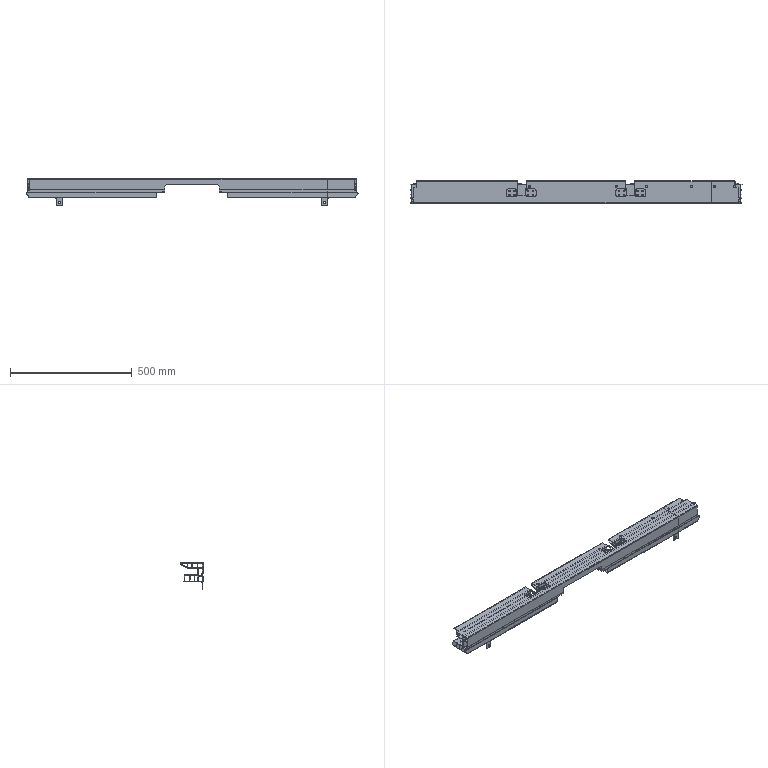NC program | NX | posted with a generic post | part box 1365 x 90.95 x 108.501 mm
Lines 10674 to 11425 of 22311:
(DRILLING , TOOL : D6A45)
N21340 T07 M6
N21342 G54
N21344 G17 G0 G90 X636.499 Y-0.225 B0. C0. S3500 M3
N21346 G43 Z30. H7
N21348 G94 G81 G98 Z-31. F250. R-27.
N21350 X600. Y0.175
N21352 X563.5
N21354 X423. Y0.725
N21356 X373.
N21358 X364.736 Y-18.525
N21360 X328. Y0.725
N21362 X314.736 Y-18.525
N21364 X278. Y0.725
N21366 X264.736 Y-18.525
N21368 X248. Y0.725
N21370 X-248.
N21372 X-264.736 Y-18.525
N21374 X-278. Y0.725
N21376 X-314.736 Y-18.525
N21378 X-328. Y0.725
N21380 X-364.736 Y-18.525
N21382 X-373. Y0.725
N21384 X-423.
N21386 X-563.501 Y-0.225
N21388 X-600. Y0.175
N21390 X-636.5
N21392 G80
N21394 G0 X-636.5 Y0.175 Z30.
(DRILLING_COPY_1 , TOOL : D6A45)
N21396 X25.103 Y-6.202
N21398 G81 Z-86.5 F250. R-82.5
N21400 G80
N21402 G0 X25.103 Y-6.202 Z30.
N21404 M5
(DRILLING_COPY , TOOL : 7.1ZT)
N21406 T17 M6
N21408 G54
N21410 G17 G0 G90 X-636.5 Y0.175 B0. C0. S1500 M3
N21412 G43 Z30. H17
N21414 G94 G83 G98 Z-36.103 F150. Q4. R-27.
N21416 X-563.501 Y-0.225
N21418 X563.5 Y0.175
N21420 X636.499 Y-0.225
N21422 G80
N21424 G0 X636.499 Y-0.225 Z30.
N21426 M5
(DRILLING_COPY_COPY , TOOL : 9.0ZT)
N21428 T19 M6
N21430 G54
N21432 G17 G0 G90 X-423. Y0.725 B0. C0. S1500 M3
N21434 G43 Z30. H19
N21436 G94 G83 G98 Z-36.704 F150. Q4. R-27.
N21438 X-373.
N21440 X-364.736 Y-18.525
N21442 X-328. Y0.725
N21444 X-314.736 Y-18.525
N21446 X-278. Y0.725
N21448 X-264.736 Y-18.525
N21450 X-248. Y0.725
N21452 X248.
N21454 X264.736 Y-18.525
N21456 X278. Y0.725
N21458 X314.736 Y-18.525
N21460 X328. Y0.725
N21462 X364.736 Y-18.525
N21464 X373. Y0.725
N21466 X423.
N21468 G80
N21470 G0 X423. Y0.725 Z30.
N21472 M5
(DRILLING_COPY_COPY_COPY , TOOL : 6.6ZT)
N21474 T14 M6
N21476 G54
N21478 G17 G0 G90 X25.103 Y-6.202 B0. C0. S1500 M3
N21480 G43 Z30. H14
N21482 G94 G83 G98 Z-91.453 F150. Q4. R-82.5
N21484 G80
N21486 G0 X25.103 Y-6.202 Z30.
N21488 M5
(FLOOR_WALL , TOOL : D10)
N21490 T10 M6
N21492 G54
N21494 G17 G0 G90 X-138.045 Y42.675 B0. C0. S6000 M3
N21496 G43 Z30. H10
N21498 Z-28.5
N21500 G94 G1 Z-30. F1000.
N21502 X-140.411 Y41.678
N21504 G3 X-139.545 Y41.178 R1.
N21506 G1 X-522.999
N21508 Y41.234
N21510 X-139.545
N21512 Y41.291
N21514 X-522.999
N21516 Y41.347
N21518 X-139.545
N21520 Y41.403
N21522 X-522.999
N21524 Y41.46
N21526 X-139.545
N21528 Y41.516
N21530 X-522.999
N21532 Y41.572
N21534 X-139.545
N21536 Y41.629
N21538 X-522.999
N21540 Y41.685
N21542 X-139.545
N21544 Y41.741
N21546 X-522.999
N21548 Y41.798
N21550 X-139.545
N21552 Y41.854
N21554 X-522.999
N21556 Y41.91
N21558 X-139.545
N21560 Y41.966
N21562 X-522.999
N21564 Y42.023
N21566 X-139.545
N21568 Y42.079
N21570 X-522.999
N21572 Y42.135
N21574 X-139.545
N21576 Y42.192
N21578 X-522.999
N21580 Y42.248
N21582 X-139.545
N21584 Y42.304
N21586 X-522.999
N21588 Y42.361
N21590 X-139.545
N21592 Y42.417
N21594 X-522.999
N21596 Y42.473
N21598 X-139.545
N21600 Y42.53
N21602 X-522.999
N21604 Y42.586
N21606 X-139.545
N21608 Y42.642
N21610 X-522.999
N21612 Y42.699
N21614 X-139.545
N21616 Y42.755
N21618 X-522.999
N21620 Y42.811
N21622 X-139.545
N21624 Y42.868
N21626 X-522.999
N21628 Y42.924
N21630 X-139.545
N21632 Y42.98
N21634 X-522.999
N21636 Y43.037
N21638 X-139.545
N21640 Y43.093
N21642 X-522.999
N21644 Y43.149
N21646 X-139.545
N21648 Y43.205
N21650 X-522.999
N21652 Y43.262
N21654 X-139.545
N21656 Y43.318
N21658 X-522.999
N21660 Y43.374
N21662 X-139.545
N21664 Y43.431
N21666 X-522.999
N21668 Y43.487
N21670 X-139.545
N21672 Y43.543
N21674 X-522.999
N21676 Y43.6
N21678 X-139.545
N21680 Y43.656
N21682 X-522.999
N21684 Y43.712
N21686 X-139.545
N21688 Y43.769
N21690 X-522.999
N21692 Y43.825
N21694 X-139.545
N21696 Y43.881
N21698 X-522.999
N21700 Y43.938
N21702 X-139.545
N21704 Y43.994
N21706 X-522.999
N21708 Y44.05
N21710 X-139.545
N21712 Y44.107
N21714 X-522.999
N21716 Y44.163
N21718 X-139.545
N21720 Y44.219
N21722 X-522.999
N21724 Y44.276
N21726 X-139.545
N21728 Y44.332
N21730 X-522.999
N21732 Y44.388
N21734 X-139.545
N21736 Y44.445
N21738 X-522.999
N21740 Y44.501
N21742 X-139.545
N21744 Y44.557
N21746 X-522.999
N21748 Y44.613
N21750 X-139.545
N21752 Y44.67
N21754 X-522.999
N21756 Y44.726
N21758 X-139.545
N21760 Y44.782
N21762 X-522.999
N21764 Y44.839
N21766 X-139.545
N21768 Y44.895
N21770 X-522.999
N21772 Y44.951
N21774 X-139.545
N21776 Y45.008
N21778 X-522.999
N21780 Y45.064
N21782 X-139.545
N21784 Y45.12
N21786 X-522.999
N21788 Y45.177
N21790 X-139.545
N21792 Y45.233
N21794 X-522.999
N21796 G3 X-522.499 Y44.367 R1.
N21798 G1 Z-28.5
N21800 G0 Z30.
N21802 X-674.702 Y46.829
N21804 Z-28.5
N21806 G1 Z-30.
N21808 X-674.068 Y45.731
N21810 G3 X-673.202 Y45.231 R1.
N21812 G1 X-566.999
N21814 Y41.175
N21816 X-673.202
N21818 G2 X-674.068 Y41.675 R1.
N21820 G1 X-674.702 Y42.773
N21822 Z-28.5
N21824 G0 Z30.
N21826 X138.164 Y46.627
N21828 Z-28.5
N21830 G1 Z-30.
N21832 X138.681 Y45.731
N21834 G3 X139.547 Y45.231 R1.
N21836 G1 X523.001
N21838 Y41.175
N21840 X139.547
N21842 G2 X138.681 Y41.675 R1.
N21844 G1 X138.047 Y42.773
N21846 Z-28.5
N21848 G0 Z30.
(FLOOR_WALL_COPY , TOOL : D10)
N21850 X110.406 Y15.475
N21852 Z-51.5
N21854 G1 Z-53.
N21856 X111.504 Y16.109
N21858 G3 X112.004 Y16.975 R1.
N21860 G1 Y47.475
N21862 X116.511
N21864 Y16.975
N21866 X121.018
N21868 Y48.975
N21870 X125.525
N21872 Y16.975
N21874 X130.033
N21876 Y48.975
N21878 X134.54
N21880 Y16.975
N21882 X139.047
N21884 Y48.975
N21886 G3 X138.547 Y49.841 R1.
N21888 G1 X137.449 Y50.475
N21890 Z-51.5
N21892 G0 Z30.
N21894 X137.949 Y15.475
N21896 Z-51.5
N21898 G1 Z-53.
N21900 X139.047 Y16.109
N21902 G3 X139.547 Y16.975 R1.
N21904 G1 Y46.046
N21906 X142.303 Y48.801
N21908 X142.451 Y48.945
N21910 G3 X142.727 Y49.906 R1.
N21912 G1 X142.453 Y51.007
N21914 Z-51.5
N21916 G0 Z30.
N21918 X95.501 Y34.652
N21920 Z-83.5
N21922 G1 Z-85.
N21924 X95.998 Y32.286
N21926 G3 X96.498 Y33.152 R1.
N21928 G1 Y17.798
N21930 X91.549
N21932 Y33.152
N21934 X86.601
N21936 Y17.798
N21938 X81.652
N21940 Y33.152
N21942 X76.703
N21944 Y17.798
N21946 X71.755
N21948 Y33.152
N21950 X66.806
N21952 Y17.798
N21954 X61.857
N21956 Y33.152
N21958 X56.909
N21960 Y17.798
N21962 X51.96
N21964 Y33.152
N21966 X47.011
N21968 Y17.798
N21970 X42.063
N21972 Y33.152
N21974 X37.114
N21976 Y17.798
N21978 X32.166
N21980 Y33.152
N21982 X27.217
N21984 Y17.798
N21986 X22.268
N21988 Y33.152
N21990 X17.32
N21992 Y17.798
N21994 X12.371
N21996 Y33.152
N21998 X7.422
N22000 Y17.798
N22002 X2.474
N22004 Y33.152
N22006 X-2.475
N22008 Y17.798
N22010 X-7.424
N22012 Y33.152
N22014 X-12.372
N22016 Y17.798
N22018 X-17.321
N22020 Y33.152
N22022 X-22.269
N22024 Y17.798
N22026 X-27.218
N22028 Y33.152
N22030 X-32.167
N22032 Y17.798
N22034 X-37.115
N22036 Y33.152
N22038 X-42.064
N22040 Y17.798
N22042 X-47.013
N22044 Y33.152
N22046 X-51.961
N22048 Y17.798
N22050 X-56.91
N22052 Y33.152
N22054 X-61.859
N22056 Y17.798
N22058 X-66.807
N22060 Y33.152
N22062 X-71.756
N22064 Y17.798
N22066 X-76.705
N22068 Y33.152
N22070 X-81.653
N22072 Y17.798
N22074 X-86.602
N22076 Y33.152
N22078 X-91.55
N22080 Y17.798
N22082 X-96.499
N22084 Y33.152
N22086 G2 X-95.999 Y34.018 R1.
N22088 G1 X-94.901 Y34.652
N22090 Z-83.5
N22092 G0 Z30.
N22094 X-95.401
N22096 Z-83.5
N22098 G1 Z-85.
N22100 X-96.499 Y34.018
N22102 G3 X-96.999 Y33.152 R1.
N22104 G1 Y17.798
N22106 G3 X-96.499 Y16.932 R1.
N22108 G1 X-95.401 Y16.298
N22110 Z-83.5
N22112 G0 Z30.
N22114 X95.403
N22116 Z-83.5
N22118 G1 Z-85.
N22120 X96.501 Y16.932
N22122 G3 X97.001 Y17.798 R1.
N22124 G1 Y33.152
N22126 G3 X96.501 Y34.018 R1.
N22128 G1 X95.403 Y34.652
N22130 Z-83.5
N22132 G0 Z30.
N22134 X95.998 Y51.975
N22136 Z-83.5
N22138 G1 Z-85.
N22140 Y49.609
N22142 G3 X96.498 Y50.475 R1.
N22144 G1 Y35.798
N22146 X91.549
N22148 Y50.475
N22150 X86.601
N22152 Y35.798
N22154 X81.652
N22156 Y50.475
N22158 X76.703
N22160 Y35.798
N22162 X71.755
N22164 Y50.475
N22166 X66.806
N22168 Y35.798
N22170 X61.857
N22172 Y50.475
N22174 X56.909
N22176 Y35.798
N22178 X51.96
N22180 Y50.475
N22182 X47.011
N22184 Y35.798
N22186 X42.063
N22188 Y50.475
N22190 X37.114
N22192 Y35.798
N22194 X32.166
N22196 Y50.475
N22198 X27.217
N22200 Y35.798
N22202 X22.268
N22204 Y50.475
N22206 X17.32
N22208 Y35.798
N22210 X12.371
N22212 Y50.475
N22214 X7.422
N22216 Y35.798
N22218 X2.474
N22220 Y50.475
N22222 X-2.475
N22224 Y35.798
N22226 X-7.424
N22228 Y50.475
N22230 X-12.372
N22232 Y35.798
N22234 X-17.321
N22236 Y50.475
N22238 X-22.269
N22240 Y35.798
N22242 X-27.218
N22244 Y50.475
N22246 X-32.167
N22248 Y35.798
N22250 X-37.115
N22252 Y50.475
N22254 X-42.064
N22256 Y35.798
N22258 X-47.013
N22260 Y50.475
N22262 X-51.961
N22264 Y35.798
N22266 X-56.91
N22268 Y50.475
N22270 X-61.859
N22272 Y35.798
N22274 X-66.807
N22276 Y50.475
N22278 X-71.756
N22280 Y35.798
N22282 X-76.705
N22284 Y50.475
N22286 X-81.653
N22288 Y35.798
N22290 X-86.602
N22292 Y50.475
N22294 X-91.55
N22296 Y35.798
N22298 X-96.499
N22300 Y50.475
N22302 G2 X-95.999 Y51.341 R1.
N22304 G1 X-94.901 Y51.975
N22306 Z-83.5
N22308 G0 Z30.
N22310 X-95.401
N22312 Z-83.5
N22314 G1 Z-85.
N22316 X-96.499 Y51.341
N22318 G3 X-96.999 Y50.475 R1.
N22320 G1 Y35.798
N22322 G3 X-96.499 Y34.932 R1.
N22324 G1 X-95.401 Y34.298
N22326 Z-83.5
N22328 G0 Z30.
N22330 X95.403
N22332 Z-83.5
N22334 G1 Z-85.
N22336 X96.501 Y34.932
N22338 G3 X97.001 Y35.798 R1.
N22340 G1 Y50.475
N22342 G3 X96.501 Y51.341 R1.
N22344 G1 X95.403 Y51.975
N22346 Z-83.5
N22348 G0 Z30.
N22350 X-684.25 Y35.972
N22352 Z-51.5
N22354 G1 Z-53.
N22356 X-683.616
N22358 G3 X-682.75 Y35.472 R1.
N22360 G1 X-675.676
N22362 Y32.475
N22364 X-682.75
N22366 G2 X-683.616 Y32.975 R1.
N22368 G1 X-684.25 Y34.073
N22370 Z-51.5
N22372 G0 Z30.
N22374 Y31.573
N22376 Z-51.5
N22378 G1 Z-53.
N22380 X-683.616 Y30.475
N22382 G3 X-682.75 Y29.975 R1.
N22384 G1 X-682.454
N22386 X-682.237 Y31.975
N22388 X-675.176
N22390 Y35.975
N22392 X-682.1
N22394 X-682.38 Y37.975
N22396 X-682.75
N22398 G3 X-683.616 Y37.475 R1.
N22400 G1 X-684.25 Y36.377
N22402 Z-51.5
N22404 G0 Z30.
N22406 X-110.404 Y48.975
N22408 Z-51.5
N22410 G1 Z-53.
N22412 X-111.502 Y48.341
N22414 G3 X-112.002 Y47.475 R1.
N22416 G1 Y16.975
N22418 X-116.509
N22420 Y47.475
N22422 X-117.999 Y48.975
N22424 X-121.016
N22426 Y16.975
N22428 X-125.524
N22430 Y48.975
N22432 X-130.031
N22434 Y16.975
N22436 X-134.538
N22438 Y48.975
N22440 X-139.045
N22442 Y16.975
N22444 G3 X-138.545 Y16.109 R1.
N22446 G1 X-137.447 Y15.475
N22448 Z-51.5
N22450 G0 Z30.
N22452 X-142.451 Y51.007
N22454 Z-51.5
N22456 G1 Z-53.
N22458 X-142.726 Y49.906
N22460 G3 X-142.45 Y48.945 R1.
N22462 G1 X-142.301 Y48.801
N22464 X-139.545 Y46.046
N22466 Y16.975
N22468 G3 X-139.045 Y16.109 R1.
N22470 G1 X-137.947 Y15.475
N22472 Z-51.5
N22474 G0 Z30.
(11 , TOOL : D10)
N22476 X-526.169 Y52.203 S5500
N22478 Z-11.
N22480 G1 Z-14. F500.
N22482 X-527.502 Y51.433
N22484 G3 X-528.001 Y50.566 R1.
N22486 G1 X-527.999 Y44.787 F1000.
N22488 Y42.175
N22490 X-527.998 Y41.827
N22492 X-528.016 Y41.759
N22494 X-527.998 Y41.744
N22496 X-528. Y40.785
N22498 Y36.728
N22500 G3 X-527.5 Y35.862 R1.
N22502 G1 X-526.18 Y35.099
N22504 Z-11.
N22506 G0 X-526.169 Y52.204 Z-22.
N22508 G1 Z-25. F500.
N22510 X-527.502 Y51.433
N22512 G3 X-528.001 Y50.566 R1.
N22514 G1 X-527.996 Y45.231 F1000.
N22516 X-527.999 Y44.787
N22518 Y42.175
N22520 X-527.996 Y41.827
N22522 X-528.015 Y41.773
N22524 X-527.996 Y41.758
N22526 X-527.998 Y40.785
N22528 X-527.999 Y36.728
N22530 G3 X-527.499 Y35.862 R1.
N22532 G1 X-526.178 Y35.099
N22534 Z-22.
N22536 G0 Z30.
N22538 X-563.83 Y35.148
N22540 Z-11.
N22542 G1 Z-14. F500.
N22544 X-562.498 Y35.917
N22546 G3 X-561.998 Y36.784 R1.
N22548 G1 X-561.999 Y42.175 F1000.
N22550 Y44.787
N22552 X-561.998 Y50.418
N22554 Y50.566
N22556 G3 X-562.494 Y51.434 R1.
N22558 G1 X-563.828 Y52.211
N22560 Z-11.
N22562 G0 X-563.831 Y35.147 Z-22.
N22564 G1 Z-25. F500.
N22566 X-562.499 Y35.917
N22568 G3 X-562. Y36.784 R1.
N22570 G1 X-562.002 Y41.758 F1000.
N22572 X-561.999 Y42.175
N22574 Y44.787
N22576 X-562.003 Y45.231
N22578 X-561.999 Y50.566
N22580 G3 X-562.498 Y51.433 R1.
N22582 G1 X-563.831 Y52.204
N22584 Z-22.
N22586 G0 Z30.
N22588 X563.831 Y52.203
N22590 Z-11.
N22592 G1 Z-14. F500.
N22594 X562.498 Y51.433
N22596 G3 X561.999 Y50.566 R1.
N22598 G1 X562.001 Y44.787 F1000.
N22600 Y42.175
N22602 X562.002 Y41.827
N22604 X561.984 Y41.759
N22606 X562.002 Y41.744
N22608 X562. Y40.785
N22610 Y36.784
N22612 G3 X562.5 Y35.918 R1.
N22614 G1 X563.832 Y35.148
N22616 Z-11.
N22618 G0 X563.831 Y52.204 Z-22.
N22620 G1 Z-25. F500.
N22622 X562.498 Y51.433
N22624 G3 X561.999 Y50.566 R1.
N22626 G1 X562.004 Y45.231 F1000.
N22628 X562.001 Y44.787
N22630 Y42.175
N22632 X562.004 Y41.827
N22634 X561.985 Y41.773
N22636 X562.004 Y41.758
N22638 X562.002 Y40.785
N22640 X562.001 Y36.784
N22642 G3 X562.501 Y35.918 R1.
N22644 G1 X563.834 Y35.148
N22646 Z-22.
N22648 G0 Z30.
N22650 X526.17
N22652 Z-11.
N22654 G1 Z-14. F500.
N22656 X527.502 Y35.917
N22658 G3 X528.002 Y36.784 R1.
N22660 G1 X528.001 Y42.175 F1000.
N22662 Y44.787
N22664 X528.002 Y50.344
N22666 Y50.566
N22668 G3 X527.505 Y51.434 R1.
N22670 G1 X526.172 Y52.208
N22672 Z-11.
N22674 G0 X526.169 Y35.147 Z-22.
N22676 G1 Z-25. F500.
N22678 X527.501 Y35.917
N22680 G3 X528. Y36.784 R1.
N22682 G1 X527.998 Y41.758 F1000.
N22684 X528.001 Y42.175
N22686 Y44.787
N22688 X527.997 Y45.231
N22690 X528.001 Y50.566
N22692 G3 X527.502 Y51.433 R1.
N22694 G1 X526.169 Y52.204
N22696 Z-22.
N22698 G0 Z30.
(11_COPY , TOOL : D10)
N22700 X105.164 Y-0.529
N22702 Z-61.
N22704 G1 Z-64. F500.
N22706 X106.502 Y0.244
N22708 G3 X107.002 Y1.11 R1.
N22710 G1 X107.001 Y21.976 F1000.
N22712 Y45.475
N22714 X107.003 Y65.34
N22716 G3 X106.503 Y66.207 R1.
N22718 G1 X105.165 Y66.979
N22720 Z-61.
N22722 G0 X105.163 Y-0.529 Z-72.
N22724 G1 Z-75. F500.
N22726 X106.501 Y0.244
N22728 G3 X107.001 Y1.11 R1.
N22730 G1 Y21.976 F1000.
N22732 Y45.475
N22734 X107.002 Y65.34
N22736 G3 X106.502 Y66.207 R1.
N22738 G1 X105.165 Y66.979
N22740 Z-72.
N22742 G0 Z30.
N22744 X-105.165
N22746 Z-61.
N22748 G1 Z-64. F500.
N22750 X-106.503 Y66.207
N22752 G3 X-107.003 Y65.34 R1.
N22754 G1 X-106.999 Y45.475 F1000.
N22756 Y21.976
N22758 X-107. Y0.998
N22760 G3 X-106.5 Y0.132 R1.
N22762 G1 X-105.186 Y-0.627
N22764 Z-61.
N22766 G0 X-105.164 Y66.979 Z-72.
N22768 G1 Z-75. F500.
N22770 X-106.502 Y66.207
N22772 G3 X-107.002 Y65.34 R1.
N22774 G1 X-106.999 Y45.475 F1000.
N22776 Y21.976
N22778 X-107. Y0.998
N22780 G3 X-106.5 Y0.132 R1.
N22782 G1 X-105.185 Y-0.627
N22784 Z-72.
N22786 G0 Z30.
N22788 M5